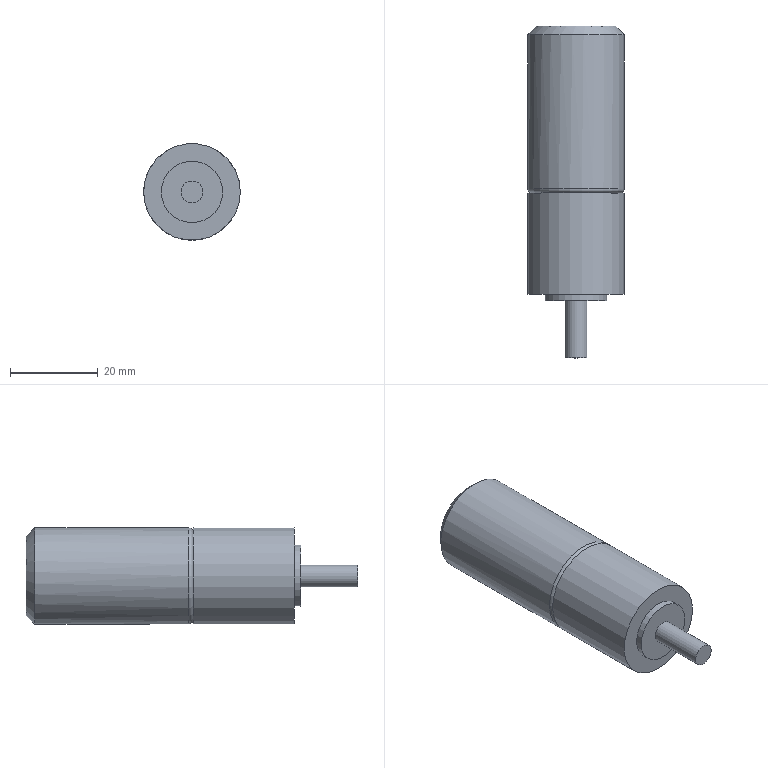Part | NX | features 5003_107_Reduction motor 2 | 1 solid | 11 faces | box 22 x 75.53 x 22 mm | volume 23541 mm3 | plane 5 | cylinder 4 | torus 1 | cone 1 | commonest cylinder face diameters 22 x2 5 x1 14 x1
STEP:
#1=CARTESIAN_POINT('',(-214.275,-568.6,-110.5));
#2=VERTEX_POINT('',#1);
#3=CARTESIAN_POINT('',(-216.775,-568.6,-110.5));
#4=DIRECTION('',(0.,-1.,0.));
#5=DIRECTION('',(1.,0.,0.));
#6=AXIS2_PLACEMENT_3D('',#3,#4,#5);
#7=CIRCLE('',#6,2.5);
#8=EDGE_CURVE('',#2,#2,#7,.T.);
#9=ORIENTED_EDGE('',*,*,#8,.T.);
#10=EDGE_LOOP('',(#9));
#11=FACE_BOUND('',#10,.T.);
#12=CARTESIAN_POINT('',(-216.775,-568.6,-110.5));
#13=DIRECTION('',(0.,1.,0.));
#14=DIRECTION('',(-1.,0.,0.));
#15=AXIS2_PLACEMENT_3D('',#12,#13,#14);
#16=PLANE('',#15);
#17=ADVANCED_FACE('',(#11),#16,.F.);
#18=ORIENTED_EDGE('',*,*,#8,.F.);
#19=EDGE_LOOP('',(#18));
#20=FACE_BOUND('',#19,.T.);
#21=CARTESIAN_POINT('',(-214.275,-555.6,-110.5));
#22=VERTEX_POINT('',#21);
#23=CARTESIAN_POINT('',(-216.775,-555.6,-110.5));
#24=DIRECTION('',(0.,-1.,0.));
#25=DIRECTION('',(1.,0.,0.));
#26=AXIS2_PLACEMENT_3D('',#23,#24,#25);
#27=CIRCLE('',#26,2.5);
#28=EDGE_CURVE('',#22,#22,#27,.T.);
#29=ORIENTED_EDGE('',*,*,#28,.T.);
#30=EDGE_LOOP('',(#29));
#31=FACE_BOUND('',#30,.T.);
#32=CARTESIAN_POINT('',(-216.775,-586.987,-110.5));
#33=DIRECTION('',(0.,-1.,0.));
#34=DIRECTION('',(1.,0.,0.));
#35=AXIS2_PLACEMENT_3D('',#32,#33,#34);
#36=CYLINDRICAL_SURFACE('',#35,2.5);
#37=ADVANCED_FACE('',(#20,#31),#36,.T.);
#38=ORIENTED_EDGE('',*,*,#28,.F.);
#39=EDGE_LOOP('',(#38));
#40=FACE_BOUND('',#39,.T.);
#41=CARTESIAN_POINT('',(-209.775,-555.6,-110.5));
#42=VERTEX_POINT('',#41);
#43=CARTESIAN_POINT('',(-216.775,-555.6,-110.5));
#44=DIRECTION('',(0.,-1.,0.));
#45=DIRECTION('',(1.,0.,0.));
#46=AXIS2_PLACEMENT_3D('',#43,#44,#45);
#47=CIRCLE('',#46,7.);
#48=EDGE_CURVE('',#42,#42,#47,.T.);
#49=ORIENTED_EDGE('',*,*,#48,.T.);
#50=EDGE_LOOP('',(#49));
#51=FACE_BOUND('',#50,.T.);
#52=CARTESIAN_POINT('',(-219.275,-555.6,-110.5));
#53=DIRECTION('',(0.,1.,0.));
#54=DIRECTION('',(-1.,0.,0.));
#55=AXIS2_PLACEMENT_3D('',#52,#53,#54);
#56=PLANE('',#55);
#57=ADVANCED_FACE('',(#40,#51),#56,.F.);
#58=ORIENTED_EDGE('',*,*,#48,.F.);
#59=EDGE_LOOP('',(#58));
#60=FACE_BOUND('',#59,.T.);
#61=CARTESIAN_POINT('',(-209.775,-554.1,-110.5));
#62=VERTEX_POINT('',#61);
#63=CARTESIAN_POINT('',(-216.775,-554.1,-110.5));
#64=DIRECTION('',(0.,-1.,0.));
#65=DIRECTION('',(1.,0.,0.));
#66=AXIS2_PLACEMENT_3D('',#63,#64,#65);
#67=CIRCLE('',#66,7.);
#68=EDGE_CURVE('',#62,#62,#67,.T.);
#69=ORIENTED_EDGE('',*,*,#68,.T.);
#70=EDGE_LOOP('',(#69));
#71=FACE_BOUND('',#70,.T.);
#72=CARTESIAN_POINT('',(-216.775,-586.987,-110.5));
#73=DIRECTION('',(0.,-1.,0.));
#74=DIRECTION('',(1.,0.,0.));
#75=AXIS2_PLACEMENT_3D('',#72,#73,#74);
#76=CYLINDRICAL_SURFACE('',#75,7.);
#77=ADVANCED_FACE('',(#60,#71),#76,.T.);
#78=ORIENTED_EDGE('',*,*,#68,.F.);
#79=EDGE_LOOP('',(#78));
#80=FACE_BOUND('',#79,.T.);
#81=CARTESIAN_POINT('',(-205.775,-554.1,-110.5));
#82=VERTEX_POINT('',#81);
#83=CARTESIAN_POINT('',(-216.775,-554.1,-110.5));
#84=DIRECTION('',(0.,-1.,0.));
#85=DIRECTION('',(1.,0.,0.));
#86=AXIS2_PLACEMENT_3D('',#83,#84,#85);
#87=CIRCLE('',#86,11.);
#88=EDGE_CURVE('',#82,#82,#87,.T.);
#89=ORIENTED_EDGE('',*,*,#88,.T.);
#90=EDGE_LOOP('',(#89));
#91=FACE_BOUND('',#90,.T.);
#92=CARTESIAN_POINT('',(-223.775,-554.1,-110.5));
#93=DIRECTION('',(0.,1.,0.));
#94=DIRECTION('',(-1.,0.,0.));
#95=AXIS2_PLACEMENT_3D('',#92,#93,#94);
#96=PLANE('',#95);
#97=ADVANCED_FACE('',(#80,#91),#96,.F.);
#98=ORIENTED_EDGE('',*,*,#88,.F.);
#99=EDGE_LOOP('',(#98));
#100=FACE_BOUND('',#99,.T.);
#101=CARTESIAN_POINT('',(-205.775,-531.07,-110.5));
#102=VERTEX_POINT('',#101);
#103=CARTESIAN_POINT('',(-216.775,-531.07,-110.5));
#104=DIRECTION('',(0.,-1.,0.));
#105=DIRECTION('',(1.,0.,0.));
#106=AXIS2_PLACEMENT_3D('',#103,#104,#105);
#107=CIRCLE('',#106,11.);
#108=EDGE_CURVE('',#102,#102,#107,.T.);
#109=ORIENTED_EDGE('',*,*,#108,.T.);
#110=EDGE_LOOP('',(#109));
#111=FACE_BOUND('',#110,.T.);
#112=CARTESIAN_POINT('',(-216.775,-586.987,-110.5));
#113=DIRECTION('',(0.,-1.,0.));
#114=DIRECTION('',(1.,0.,0.));
#115=AXIS2_PLACEMENT_3D('',#112,#113,#114);
#116=CYLINDRICAL_SURFACE('',#115,11.);
#117=ADVANCED_FACE('',(#100,#111),#116,.T.);
#118=ORIENTED_EDGE('',*,*,#108,.F.);
#119=EDGE_LOOP('',(#118));
#120=FACE_BOUND('',#119,.T.);
#121=CARTESIAN_POINT('',(-206.775,-531.07,-110.5));
#122=VERTEX_POINT('',#121);
#123=CARTESIAN_POINT('',(-216.775,-531.07,-110.5));
#124=DIRECTION('',(0.,-1.,0.));
#125=DIRECTION('',(1.,0.,0.));
#126=AXIS2_PLACEMENT_3D('',#123,#124,#125);
#127=CIRCLE('',#126,10.);
#128=EDGE_CURVE('',#122,#122,#127,.T.);
#129=ORIENTED_EDGE('',*,*,#128,.T.);
#130=EDGE_LOOP('',(#129));
#131=FACE_BOUND('',#130,.T.);
#132=CARTESIAN_POINT('',(-226.775,-531.07,-110.5));
#133=DIRECTION('',(0.,-1.,0.));
#134=DIRECTION('',(1.,0.,0.));
#135=AXIS2_PLACEMENT_3D('',#132,#133,#134);
#136=PLANE('',#135);
#137=ADVANCED_FACE('',(#120,#131),#136,.F.);
#138=ORIENTED_EDGE('',*,*,#128,.F.);
#139=EDGE_LOOP('',(#138));
#140=FACE_BOUND('',#139,.T.);
#141=CARTESIAN_POINT('',(-205.775,-530.07,-110.5));
#142=VERTEX_POINT('',#141);
#143=CARTESIAN_POINT('',(-216.775,-530.07,-110.5));
#144=DIRECTION('',(0.,-1.,0.));
#145=DIRECTION('',(1.,0.,0.));
#146=AXIS2_PLACEMENT_3D('',#143,#144,#145);
#147=CIRCLE('',#146,11.);
#148=EDGE_CURVE('',#142,#142,#147,.T.);
#149=ORIENTED_EDGE('',*,*,#148,.T.);
#150=EDGE_LOOP('',(#149));
#151=FACE_BOUND('',#150,.T.);
#152=CARTESIAN_POINT('',(-216.775,-530.07,-110.5));
#153=DIRECTION('',(0.,-1.,0.));
#154=DIRECTION('',(1.,0.,0.));
#155=AXIS2_PLACEMENT_3D('',#152,#153,#154);
#156=TOROIDAL_SURFACE('',#155,10.,1.);
#157=ADVANCED_FACE('',(#140,#151),#156,.T.);
#158=CARTESIAN_POINT('',(-216.775,-495.07,-121.5));
#159=VERTEX_POINT('',#158);
#160=CARTESIAN_POINT('',(-216.775,-495.07,-110.5));
#161=DIRECTION('',(0.,-1.,0.));
#162=DIRECTION('',(0.,0.,-1.));
#163=AXIS2_PLACEMENT_3D('',#160,#161,#162);
#164=CIRCLE('',#163,11.);
#165=EDGE_CURVE('',#159,#159,#164,.T.);
#166=ORIENTED_EDGE('',*,*,#165,.T.);
#167=EDGE_LOOP('',(#166));
#168=FACE_BOUND('',#167,.T.);
#169=ORIENTED_EDGE('',*,*,#148,.F.);
#170=EDGE_LOOP('',(#169));
#171=FACE_BOUND('',#170,.T.);
#172=CARTESIAN_POINT('',(-216.775,-586.987,-110.5));
#173=DIRECTION('',(0.,-1.,0.));
#174=DIRECTION('',(1.,0.,0.));
#175=AXIS2_PLACEMENT_3D('',#172,#173,#174);
#176=CYLINDRICAL_SURFACE('',#175,11.);
#177=ADVANCED_FACE('',(#168,#171),#176,.T.);
#178=CARTESIAN_POINT('',(-216.775,-493.07,-119.5));
#179=VERTEX_POINT('',#178);
#180=CARTESIAN_POINT('',(-216.775,-493.07,-110.5));
#181=DIRECTION('',(0.,-1.,0.));
#182=DIRECTION('',(0.,0.,-1.));
#183=AXIS2_PLACEMENT_3D('',#180,#181,#182);
#184=CIRCLE('',#183,9.);
#185=EDGE_CURVE('',#179,#179,#184,.F.);
#186=ORIENTED_EDGE('',*,*,#185,.T.);
#187=EDGE_LOOP('',(#186));
#188=FACE_BOUND('',#187,.T.);
#189=CARTESIAN_POINT('',(-227.775,-493.07,-110.5));
#190=DIRECTION('',(0.,-1.,0.));
#191=DIRECTION('',(1.,0.,0.));
#192=AXIS2_PLACEMENT_3D('',#189,#190,#191);
#193=PLANE('',#192);
#194=ADVANCED_FACE('',(#188),#193,.F.);
#195=ORIENTED_EDGE('',*,*,#185,.F.);
#196=EDGE_LOOP('',(#195));
#197=FACE_BOUND('',#196,.T.);
#198=ORIENTED_EDGE('',*,*,#165,.F.);
#199=EDGE_LOOP('',(#198));
#200=FACE_BOUND('',#199,.T.);
#201=CARTESIAN_POINT('',(-216.775,-495.07,-110.5));
#202=DIRECTION('',(0.,-1.,0.));
#203=DIRECTION('',(0.,0.,-1.));
#204=AXIS2_PLACEMENT_3D('',#201,#202,#203);
#205=CONICAL_SURFACE('',#204,11.,0.7854);
#206=ADVANCED_FACE('',(#197,#200),#205,.T.);
#207=CLOSED_SHELL('',(#17,#37,#57,#77,#97,#117,#137,#157,#177,#194,#206));
#208=MANIFOLD_SOLID_BREP('',#207);
#209=(LENGTH_UNIT()NAMED_UNIT(*)SI_UNIT(.MILLI.,.METRE.));
#210=UNCERTAINTY_MEASURE_WITH_UNIT(LENGTH_MEASURE(0.00001),#209,'','');
#211=(NAMED_UNIT(*)PLANE_ANGLE_UNIT()SI_UNIT($,.RADIAN.));
#212=(NAMED_UNIT(*)SI_UNIT($,.STERADIAN.)SOLID_ANGLE_UNIT());
#213=(GEOMETRIC_REPRESENTATION_CONTEXT(3)GLOBAL_UNCERTAINTY_ASSIGNED_CONTEXT((#210))GLOBAL_UNIT_ASSIGNED_CONTEXT((#209,#211,#212))REPRESENTATION_CONTEXT('',''));
#214=ADVANCED_BREP_SHAPE_REPRESENTATION('',(#208),#213);